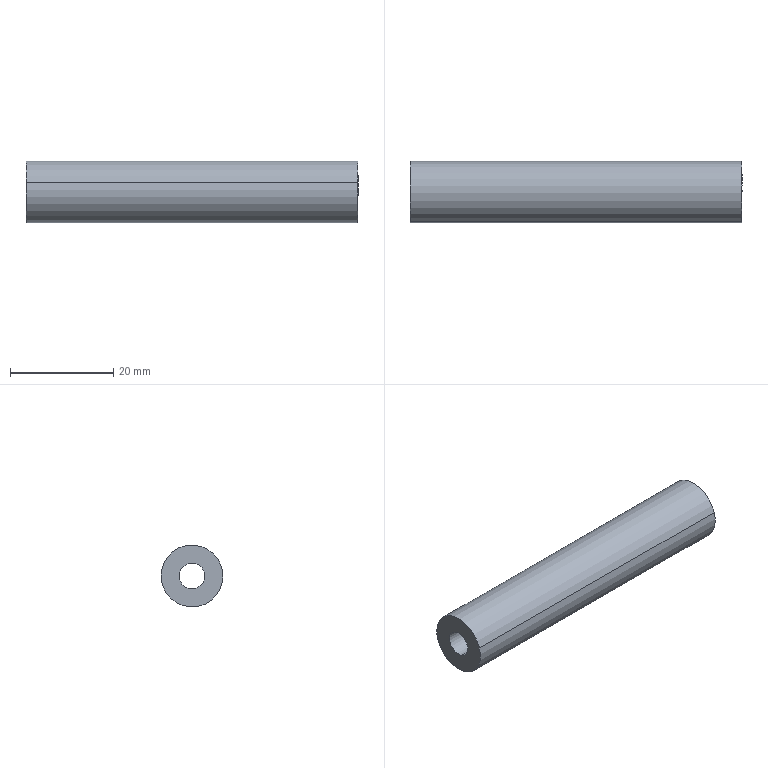Part | STEP file | Completa.sldasm-Part-5_Valor predeterminado | 1 solid | 6 faces | box 64.439 x 12 x 12 mm | volume 6023 mm3 | cylinder 4 | plane 2 | commonest cylinder face diameters 5 x2 12 x2
STEP:
#1=CARTESIAN_POINT('',(0.,0.,0.));
#2=DIRECTION('',(0.,0.,1.));
#3=DIRECTION('',(1.,0.,0.));
#4=AXIS2_PLACEMENT_3D('',#1,#2,#3);
#5=CARTESIAN_POINT('',(-262.606,26.635,-33.219));
#6=VERTEX_POINT('',#5);
#7=CARTESIAN_POINT('',(-198.167,26.635,-33.219));
#8=VERTEX_POINT('',#7);
#9=CARTESIAN_POINT('',(-262.606,26.635,-33.219));
#10=DIRECTION('',(1.,0.,0.));
#11=VECTOR('',#10,1.);
#12=LINE('',#9,#11);
#13=CARTESIAN_POINT('',(-262.606,25.863,-35.597));
#14=DIRECTION('',(1.,0.,0.));
#15=DIRECTION('',(0.,0.309,0.9511));
#16=AXIS2_PLACEMENT_3D('',#13,#14,#15);
#17=CYLINDRICAL_SURFACE('',#16,2.5);
#18=CARTESIAN_POINT('',(6.283,0.));
#19=DIRECTION('',(0.,1.));
#20=VECTOR('',#19,1.);
#21=LINE('',#18,#20);
#22=(GEOMETRIC_REPRESENTATION_CONTEXT(2)PARAMETRIC_REPRESENTATION_CONTEXT()REPRESENTATION_CONTEXT('',''));
#23=DEFINITIONAL_REPRESENTATION('',(#21),#22);
#24=PCURVE('',#17,#23);
#25=CARTESIAN_POINT('',(-262.606,25.863,-35.597));
#26=DIRECTION('',(1.,0.,0.));
#27=DIRECTION('',(0.,0.309,0.9511));
#28=AXIS2_PLACEMENT_3D('',#25,#26,#27);
#29=CYLINDRICAL_SURFACE('',#28,2.5);
#30=CARTESIAN_POINT('',(0.,0.));
#31=DIRECTION('',(0.,1.));
#32=VECTOR('',#31,1.);
#33=LINE('',#30,#32);
#34=(GEOMETRIC_REPRESENTATION_CONTEXT(2)PARAMETRIC_REPRESENTATION_CONTEXT()REPRESENTATION_CONTEXT('',''));
#35=DEFINITIONAL_REPRESENTATION('',(#33),#34);
#36=PCURVE('',#29,#35);
#37=SURFACE_CURVE('',#12,(#24,#36),.PCURVE_S1.);
#38=EDGE_CURVE('',#6,#8,#37,.T.);
#39=ORIENTED_EDGE('',*,*,#38,.T.);
#40=CARTESIAN_POINT('',(-198.167,25.09,-37.974));
#41=VERTEX_POINT('',#40);
#42=CARTESIAN_POINT('',(-198.167,25.863,-35.597));
#43=DIRECTION('',(-1.,0.,0.));
#44=DIRECTION('',(0.,-0.309,-0.9511));
#45=AXIS2_PLACEMENT_3D('',#42,#43,#44);
#46=CIRCLE('',#45,2.5);
#47=CARTESIAN_POINT('',(9.425,64.439));
#48=DIRECTION('',(-1.,0.));
#49=VECTOR('',#48,1.);
#50=LINE('',#47,#49);
#51=(GEOMETRIC_REPRESENTATION_CONTEXT(2)PARAMETRIC_REPRESENTATION_CONTEXT()REPRESENTATION_CONTEXT('',''));
#52=DEFINITIONAL_REPRESENTATION('',(#50),#51);
#53=PCURVE('',#17,#52);
#54=CARTESIAN_POINT('',(-198.167,-9.156,-28.181));
#55=DIRECTION('',(1.,0.,0.));
#56=DIRECTION('',(0.,0.9511,-0.309));
#57=AXIS2_PLACEMENT_3D('',#54,#55,#56);
#58=PLANE('',#57);
#59=CARTESIAN_POINT('',(35.597,1.268));
#60=CARTESIAN_POINT('',(31.267,1.268));
#61=CARTESIAN_POINT('',(33.432,5.018));
#62=CARTESIAN_POINT('',(35.597,8.768));
#63=CARTESIAN_POINT('',(37.762,5.018));
#64=CARTESIAN_POINT('',(39.927,1.268));
#65=CARTESIAN_POINT('',(35.597,1.268));
#66=(BOUNDED_CURVE()B_SPLINE_CURVE(2,(#59,#60,#61,#62,#63,#64,#65),.UNSPECIFIED.,.T.,.F.)B_SPLINE_CURVE_WITH_KNOTS((1,2,2,2,2,1),(-2.094,0.,2.094,4.189,6.283,8.378),.UNSPECIFIED.)CURVE()GEOMETRIC_REPRESENTATION_ITEM()RATIONAL_B_SPLINE_CURVE((1.,0.5,1.,0.5,1.,0.5,1.))REPRESENTATION_ITEM(''));
#67=(GEOMETRIC_REPRESENTATION_CONTEXT(2)PARAMETRIC_REPRESENTATION_CONTEXT()REPRESENTATION_CONTEXT('',''));
#68=DEFINITIONAL_REPRESENTATION('',(#66),#67);
#69=PCURVE('',#58,#68);
#70=SURFACE_CURVE('',#46,(#53,#69),.PCURVE_S1.);
#71=EDGE_CURVE('',#8,#41,#70,.T.);
#72=ORIENTED_EDGE('',*,*,#71,.T.);
#73=CARTESIAN_POINT('',(-262.606,25.09,-37.974));
#74=VERTEX_POINT('',#73);
#75=CARTESIAN_POINT('',(-262.606,25.09,-37.974));
#76=DIRECTION('',(1.,0.,0.));
#77=VECTOR('',#76,1.);
#78=LINE('',#75,#77);
#79=CARTESIAN_POINT('',(3.142,0.));
#80=DIRECTION('',(0.,1.));
#81=VECTOR('',#80,1.);
#82=LINE('',#79,#81);
#83=(GEOMETRIC_REPRESENTATION_CONTEXT(2)PARAMETRIC_REPRESENTATION_CONTEXT()REPRESENTATION_CONTEXT('',''));
#84=DEFINITIONAL_REPRESENTATION('',(#82),#83);
#85=PCURVE('',#17,#84);
#86=CARTESIAN_POINT('',(3.142,0.));
#87=DIRECTION('',(0.,1.));
#88=VECTOR('',#87,1.);
#89=LINE('',#86,#88);
#90=(GEOMETRIC_REPRESENTATION_CONTEXT(2)PARAMETRIC_REPRESENTATION_CONTEXT()REPRESENTATION_CONTEXT('',''));
#91=DEFINITIONAL_REPRESENTATION('',(#89),#90);
#92=PCURVE('',#29,#91);
#93=SURFACE_CURVE('',#78,(#85,#92),.PCURVE_S1.);
#94=EDGE_CURVE('',#74,#41,#93,.T.);
#95=ORIENTED_EDGE('',*,*,#94,.F.);
#96=CARTESIAN_POINT('',(-262.606,25.863,-35.597));
#97=DIRECTION('',(-1.,0.,0.));
#98=DIRECTION('',(0.,-0.309,-0.9511));
#99=AXIS2_PLACEMENT_3D('',#96,#97,#98);
#100=CIRCLE('',#99,2.5);
#101=CARTESIAN_POINT('',(9.425,0.));
#102=DIRECTION('',(-1.,0.));
#103=VECTOR('',#102,1.);
#104=LINE('',#101,#103);
#105=(GEOMETRIC_REPRESENTATION_CONTEXT(2)PARAMETRIC_REPRESENTATION_CONTEXT()REPRESENTATION_CONTEXT('',''));
#106=DEFINITIONAL_REPRESENTATION('',(#104),#105);
#107=PCURVE('',#17,#106);
#108=CARTESIAN_POINT('',(-262.606,25.863,-35.597));
#109=DIRECTION('',(1.,0.,0.));
#110=DIRECTION('',(0.,0.9511,-0.309));
#111=AXIS2_PLACEMENT_3D('',#108,#109,#110);
#112=PLANE('',#111);
#113=CARTESIAN_POINT('',(0.,-2.5));
#114=CARTESIAN_POINT('',(-4.33,-2.5));
#115=CARTESIAN_POINT('',(-2.165,1.25));
#116=CARTESIAN_POINT('',(0.,5.));
#117=CARTESIAN_POINT('',(2.165,1.25));
#118=CARTESIAN_POINT('',(4.33,-2.5));
#119=CARTESIAN_POINT('',(0.,-2.5));
#120=(BOUNDED_CURVE()B_SPLINE_CURVE(2,(#113,#114,#115,#116,#117,#118,#119),.UNSPECIFIED.,.T.,.F.)B_SPLINE_CURVE_WITH_KNOTS((1,2,2,2,2,1),(-2.094,0.,2.094,4.189,6.283,8.378),.UNSPECIFIED.)CURVE()GEOMETRIC_REPRESENTATION_ITEM()RATIONAL_B_SPLINE_CURVE((1.,0.5,1.,0.5,1.,0.5,1.))REPRESENTATION_ITEM(''));
#121=(GEOMETRIC_REPRESENTATION_CONTEXT(2)PARAMETRIC_REPRESENTATION_CONTEXT()REPRESENTATION_CONTEXT('',''));
#122=DEFINITIONAL_REPRESENTATION('',(#120),#121);
#123=PCURVE('',#112,#122);
#124=SURFACE_CURVE('',#100,(#107,#123),.PCURVE_S1.);
#125=EDGE_CURVE('',#6,#74,#124,.T.);
#126=ORIENTED_EDGE('',*,*,#125,.F.);
#127=EDGE_LOOP('',(#39,#72,#95,#126));
#128=FACE_BOUND('',#127,.F.);
#129=ADVANCED_FACE('',(#128),#17,.F.);
#130=CARTESIAN_POINT('',(-198.167,31.569,-37.451));
#131=VERTEX_POINT('',#130);
#132=CARTESIAN_POINT('',(-198.167,20.156,-33.743));
#133=VERTEX_POINT('',#132);
#134=CARTESIAN_POINT('',(-198.167,25.863,-35.597));
#135=DIRECTION('',(1.,0.,0.));
#136=DIRECTION('',(0.,0.9511,-0.309));
#137=AXIS2_PLACEMENT_3D('',#134,#135,#136);
#138=CIRCLE('',#137,6.);
#139=CARTESIAN_POINT('',(-72.606,25.863,-35.597));
#140=DIRECTION('',(-1.,0.,0.));
#141=DIRECTION('',(0.,-0.9511,0.309));
#142=AXIS2_PLACEMENT_3D('',#139,#140,#141);
#143=CYLINDRICAL_SURFACE('',#142,6.);
#144=CARTESIAN_POINT('',(3.142,125.561));
#145=DIRECTION('',(-1.,0.));
#146=VECTOR('',#145,1.);
#147=LINE('',#144,#146);
#148=(GEOMETRIC_REPRESENTATION_CONTEXT(2)PARAMETRIC_REPRESENTATION_CONTEXT()REPRESENTATION_CONTEXT('',''));
#149=DEFINITIONAL_REPRESENTATION('',(#147),#148);
#150=PCURVE('',#143,#149);
#151=CARTESIAN_POINT('',(35.597,3.768));
#152=DIRECTION('',(1.,0.));
#153=AXIS2_PLACEMENT_2D('',#151,#152);
#154=CIRCLE('',#153,6.);
#155=(GEOMETRIC_REPRESENTATION_CONTEXT(2)PARAMETRIC_REPRESENTATION_CONTEXT()REPRESENTATION_CONTEXT('',''));
#156=DEFINITIONAL_REPRESENTATION('',(#154),#155);
#157=PCURVE('',#58,#156);
#158=SURFACE_CURVE('',#138,(#150,#157),.PCURVE_S1.);
#159=EDGE_CURVE('',#131,#133,#158,.T.);
#160=ORIENTED_EDGE('',*,*,#159,.F.);
#161=CARTESIAN_POINT('',(-262.606,31.569,-37.451));
#162=VERTEX_POINT('',#161);
#163=CARTESIAN_POINT('',(-72.606,31.569,-37.451));
#164=DIRECTION('',(-1.,0.,0.));
#165=VECTOR('',#164,1.);
#166=LINE('',#163,#165);
#167=CARTESIAN_POINT('',(3.142,0.));
#168=DIRECTION('',(0.,1.));
#169=VECTOR('',#168,1.);
#170=LINE('',#167,#169);
#171=(GEOMETRIC_REPRESENTATION_CONTEXT(2)PARAMETRIC_REPRESENTATION_CONTEXT()REPRESENTATION_CONTEXT('',''));
#172=DEFINITIONAL_REPRESENTATION('',(#170),#171);
#173=PCURVE('',#143,#172);
#174=CARTESIAN_POINT('',(-72.606,25.863,-35.597));
#175=DIRECTION('',(-1.,0.,0.));
#176=DIRECTION('',(0.,-0.9511,0.309));
#177=AXIS2_PLACEMENT_3D('',#174,#175,#176);
#178=CYLINDRICAL_SURFACE('',#177,6.);
#179=CARTESIAN_POINT('',(3.142,0.));
#180=DIRECTION('',(0.,1.));
#181=VECTOR('',#180,1.);
#182=LINE('',#179,#181);
#183=(GEOMETRIC_REPRESENTATION_CONTEXT(2)PARAMETRIC_REPRESENTATION_CONTEXT()REPRESENTATION_CONTEXT('',''));
#184=DEFINITIONAL_REPRESENTATION('',(#182),#183);
#185=PCURVE('',#178,#184);
#186=SURFACE_CURVE('',#166,(#173,#185),.PCURVE_S1.);
#187=EDGE_CURVE('',#131,#162,#186,.T.);
#188=ORIENTED_EDGE('',*,*,#187,.T.);
#189=CARTESIAN_POINT('',(-262.606,20.156,-33.743));
#190=VERTEX_POINT('',#189);
#191=CARTESIAN_POINT('',(-262.606,25.863,-35.597));
#192=DIRECTION('',(1.,0.,0.));
#193=DIRECTION('',(0.,-0.9511,0.309));
#194=AXIS2_PLACEMENT_3D('',#191,#192,#193);
#195=CIRCLE('',#194,6.);
#196=CARTESIAN_POINT('',(6.283,190.));
#197=DIRECTION('',(-1.,0.));
#198=VECTOR('',#197,1.);
#199=LINE('',#196,#198);
#200=(GEOMETRIC_REPRESENTATION_CONTEXT(2)PARAMETRIC_REPRESENTATION_CONTEXT()REPRESENTATION_CONTEXT('',''));
#201=DEFINITIONAL_REPRESENTATION('',(#199),#200);
#202=PCURVE('',#143,#201);
#203=CARTESIAN_POINT('',(0.,0.));
#204=DIRECTION('',(-1.,0.));
#205=AXIS2_PLACEMENT_2D('',#203,#204);
#206=CIRCLE('',#205,6.);
#207=(GEOMETRIC_REPRESENTATION_CONTEXT(2)PARAMETRIC_REPRESENTATION_CONTEXT()REPRESENTATION_CONTEXT('',''));
#208=DEFINITIONAL_REPRESENTATION('',(#206),#207);
#209=PCURVE('',#112,#208);
#210=SURFACE_CURVE('',#195,(#202,#209),.PCURVE_S1.);
#211=EDGE_CURVE('',#162,#190,#210,.T.);
#212=ORIENTED_EDGE('',*,*,#211,.T.);
#213=CARTESIAN_POINT('',(-72.606,20.156,-33.743));
#214=DIRECTION('',(-1.,0.,0.));
#215=VECTOR('',#214,1.);
#216=LINE('',#213,#215);
#217=CARTESIAN_POINT('',(0.,0.));
#218=DIRECTION('',(0.,1.));
#219=VECTOR('',#218,1.);
#220=LINE('',#217,#219);
#221=(GEOMETRIC_REPRESENTATION_CONTEXT(2)PARAMETRIC_REPRESENTATION_CONTEXT()REPRESENTATION_CONTEXT('',''));
#222=DEFINITIONAL_REPRESENTATION('',(#220),#221);
#223=PCURVE('',#143,#222);
#224=CARTESIAN_POINT('',(6.283,0.));
#225=DIRECTION('',(0.,1.));
#226=VECTOR('',#225,1.);
#227=LINE('',#224,#226);
#228=(GEOMETRIC_REPRESENTATION_CONTEXT(2)PARAMETRIC_REPRESENTATION_CONTEXT()REPRESENTATION_CONTEXT('',''));
#229=DEFINITIONAL_REPRESENTATION('',(#227),#228);
#230=PCURVE('',#178,#229);
#231=SURFACE_CURVE('',#216,(#223,#230),.PCURVE_S1.);
#232=EDGE_CURVE('',#133,#190,#231,.T.);
#233=ORIENTED_EDGE('',*,*,#232,.F.);
#234=EDGE_LOOP('',(#160,#188,#212,#233));
#235=FACE_BOUND('',#234,.T.);
#236=ADVANCED_FACE('',(#235),#143,.T.);
#237=CARTESIAN_POINT('',(-262.606,25.863,-35.597));
#238=DIRECTION('',(1.,0.,0.));
#239=DIRECTION('',(0.,-0.9511,0.309));
#240=AXIS2_PLACEMENT_3D('',#237,#238,#239);
#241=CIRCLE('',#240,6.);
#242=CARTESIAN_POINT('',(0.,0.));
#243=DIRECTION('',(-1.,0.));
#244=AXIS2_PLACEMENT_2D('',#242,#243);
#245=CIRCLE('',#244,6.);
#246=(GEOMETRIC_REPRESENTATION_CONTEXT(2)PARAMETRIC_REPRESENTATION_CONTEXT()REPRESENTATION_CONTEXT('',''));
#247=DEFINITIONAL_REPRESENTATION('',(#245),#246);
#248=PCURVE('',#112,#247);
#249=CARTESIAN_POINT('',(6.283,190.));
#250=DIRECTION('',(-1.,0.));
#251=VECTOR('',#250,1.);
#252=LINE('',#249,#251);
#253=(GEOMETRIC_REPRESENTATION_CONTEXT(2)PARAMETRIC_REPRESENTATION_CONTEXT()REPRESENTATION_CONTEXT('',''));
#254=DEFINITIONAL_REPRESENTATION('',(#252),#253);
#255=PCURVE('',#178,#254);
#256=SURFACE_CURVE('',#241,(#248,#255),.PCURVE_S1.);
#257=EDGE_CURVE('',#190,#162,#256,.T.);
#258=ORIENTED_EDGE('',*,*,#257,.F.);
#259=ORIENTED_EDGE('',*,*,#211,.F.);
#260=EDGE_LOOP('',(#258,#259));
#261=FACE_BOUND('',#260,.T.);
#262=ORIENTED_EDGE('',*,*,#125,.F.);
#263=CARTESIAN_POINT('',(-262.606,25.863,-35.597));
#264=DIRECTION('',(-1.,0.,0.));
#265=DIRECTION('',(0.,-0.309,-0.9511));
#266=AXIS2_PLACEMENT_3D('',#263,#264,#265);
#267=CIRCLE('',#266,2.5);
#268=CARTESIAN_POINT('',(0.,-2.5));
#269=CARTESIAN_POINT('',(-4.33,-2.5));
#270=CARTESIAN_POINT('',(-2.165,1.25));
#271=CARTESIAN_POINT('',(0.,5.));
#272=CARTESIAN_POINT('',(2.165,1.25));
#273=CARTESIAN_POINT('',(4.33,-2.5));
#274=CARTESIAN_POINT('',(0.,-2.5));
#275=(BOUNDED_CURVE()B_SPLINE_CURVE(2,(#268,#269,#270,#271,#272,#273,#274),.UNSPECIFIED.,.T.,.F.)B_SPLINE_CURVE_WITH_KNOTS((1,2,2,2,2,1),(-2.094,0.,2.094,4.189,6.283,8.378),.UNSPECIFIED.)CURVE()GEOMETRIC_REPRESENTATION_ITEM()RATIONAL_B_SPLINE_CURVE((1.,0.5,1.,0.5,1.,0.5,1.))REPRESENTATION_ITEM(''));
#276=(GEOMETRIC_REPRESENTATION_CONTEXT(2)PARAMETRIC_REPRESENTATION_CONTEXT()REPRESENTATION_CONTEXT('',''));
#277=DEFINITIONAL_REPRESENTATION('',(#275),#276);
#278=PCURVE('',#112,#277);
#279=CARTESIAN_POINT('',(3.142,0.));
#280=DIRECTION('',(-1.,0.));
#281=VECTOR('',#280,1.);
#282=LINE('',#279,#281);
#283=(GEOMETRIC_REPRESENTATION_CONTEXT(2)PARAMETRIC_REPRESENTATION_CONTEXT()REPRESENTATION_CONTEXT('',''));
#284=DEFINITIONAL_REPRESENTATION('',(#282),#283);
#285=PCURVE('',#29,#284);
#286=SURFACE_CURVE('',#267,(#278,#285),.PCURVE_S1.);
#287=EDGE_CURVE('',#74,#6,#286,.T.);
#288=ORIENTED_EDGE('',*,*,#287,.F.);
#289=EDGE_LOOP('',(#262,#288));
#290=FACE_BOUND('',#289,.T.);
#291=ADVANCED_FACE('',(#261,#290),#112,.F.);
#292=CARTESIAN_POINT('',(-198.167,25.863,-35.597));
#293=DIRECTION('',(1.,0.,0.));
#294=DIRECTION('',(0.,0.9511,-0.309));
#295=AXIS2_PLACEMENT_3D('',#292,#293,#294);
#296=CIRCLE('',#295,6.);
#297=CARTESIAN_POINT('',(35.597,3.768));
#298=DIRECTION('',(1.,0.));
#299=AXIS2_PLACEMENT_2D('',#297,#298);
#300=CIRCLE('',#299,6.);
#301=(GEOMETRIC_REPRESENTATION_CONTEXT(2)PARAMETRIC_REPRESENTATION_CONTEXT()REPRESENTATION_CONTEXT('',''));
#302=DEFINITIONAL_REPRESENTATION('',(#300),#301);
#303=PCURVE('',#58,#302);
#304=CARTESIAN_POINT('',(9.425,125.561));
#305=DIRECTION('',(-1.,0.));
#306=VECTOR('',#305,1.);
#307=LINE('',#304,#306);
#308=(GEOMETRIC_REPRESENTATION_CONTEXT(2)PARAMETRIC_REPRESENTATION_CONTEXT()REPRESENTATION_CONTEXT('',''));
#309=DEFINITIONAL_REPRESENTATION('',(#307),#308);
#310=PCURVE('',#178,#309);
#311=SURFACE_CURVE('',#296,(#303,#310),.PCURVE_S1.);
#312=EDGE_CURVE('',#133,#131,#311,.T.);
#313=ORIENTED_EDGE('',*,*,#312,.T.);
#314=ORIENTED_EDGE('',*,*,#159,.T.);
#315=EDGE_LOOP('',(#313,#314));
#316=FACE_BOUND('',#315,.T.);
#317=ORIENTED_EDGE('',*,*,#71,.T.);
#318=CARTESIAN_POINT('',(-198.167,25.863,-35.597));
#319=DIRECTION('',(-1.,0.,0.));
#320=DIRECTION('',(0.,-0.309,-0.9511));
#321=AXIS2_PLACEMENT_3D('',#318,#319,#320);
#322=CIRCLE('',#321,2.5);
#323=CARTESIAN_POINT('',(35.597,1.268));
#324=CARTESIAN_POINT('',(31.267,1.268));
#325=CARTESIAN_POINT('',(33.432,5.018));
#326=CARTESIAN_POINT('',(35.597,8.768));
#327=CARTESIAN_POINT('',(37.762,5.018));
#328=CARTESIAN_POINT('',(39.927,1.268));
#329=CARTESIAN_POINT('',(35.597,1.268));
#330=(BOUNDED_CURVE()B_SPLINE_CURVE(2,(#323,#324,#325,#326,#327,#328,#329),.UNSPECIFIED.,.T.,.F.)B_SPLINE_CURVE_WITH_KNOTS((1,2,2,2,2,1),(-2.094,0.,2.094,4.189,6.283,8.378),.UNSPECIFIED.)CURVE()GEOMETRIC_REPRESENTATION_ITEM()RATIONAL_B_SPLINE_CURVE((1.,0.5,1.,0.5,1.,0.5,1.))REPRESENTATION_ITEM(''));
#331=(GEOMETRIC_REPRESENTATION_CONTEXT(2)PARAMETRIC_REPRESENTATION_CONTEXT()REPRESENTATION_CONTEXT('',''));
#332=DEFINITIONAL_REPRESENTATION('',(#330),#331);
#333=PCURVE('',#58,#332);
#334=CARTESIAN_POINT('',(3.142,64.439));
#335=DIRECTION('',(-1.,0.));
#336=VECTOR('',#335,1.);
#337=LINE('',#334,#336);
#338=(GEOMETRIC_REPRESENTATION_CONTEXT(2)PARAMETRIC_REPRESENTATION_CONTEXT()REPRESENTATION_CONTEXT('',''));
#339=DEFINITIONAL_REPRESENTATION('',(#337),#338);
#340=PCURVE('',#29,#339);
#341=SURFACE_CURVE('',#322,(#333,#340),.PCURVE_S1.);
#342=EDGE_CURVE('',#41,#8,#341,.T.);
#343=ORIENTED_EDGE('',*,*,#342,.T.);
#344=EDGE_LOOP('',(#317,#343));
#345=FACE_BOUND('',#344,.T.);
#346=ADVANCED_FACE('',(#316,#345),#58,.T.);
#347=ORIENTED_EDGE('',*,*,#187,.F.);
#348=ORIENTED_EDGE('',*,*,#312,.F.);
#349=ORIENTED_EDGE('',*,*,#232,.T.);
#350=ORIENTED_EDGE('',*,*,#257,.T.);
#351=EDGE_LOOP('',(#347,#348,#349,#350));
#352=FACE_BOUND('',#351,.T.);
#353=ADVANCED_FACE('',(#352),#178,.T.);
#354=ORIENTED_EDGE('',*,*,#342,.T.);
#355=ORIENTED_EDGE('',*,*,#38,.F.);
#356=ORIENTED_EDGE('',*,*,#287,.F.);
#357=ORIENTED_EDGE('',*,*,#94,.T.);
#358=EDGE_LOOP('',(#354,#355,#356,#357));
#359=FACE_BOUND('',#358,.F.);
#360=ADVANCED_FACE('',(#359),#29,.F.);
#361=CLOSED_SHELL('',(#129,#236,#291,#346,#353,#360));
#362=MANIFOLD_SOLID_BREP('',#361);
#363=(LENGTH_UNIT()NAMED_UNIT(*)SI_UNIT(.MILLI.,.METRE.));
#364=UNCERTAINTY_MEASURE_WITH_UNIT(LENGTH_MEASURE(0.0000001),#363,'','');
#365=(NAMED_UNIT(*)PLANE_ANGLE_UNIT()SI_UNIT($,.RADIAN.));
#366=(NAMED_UNIT(*)SI_UNIT($,.STERADIAN.)SOLID_ANGLE_UNIT());
#367=(GEOMETRIC_REPRESENTATION_CONTEXT(3)GLOBAL_UNCERTAINTY_ASSIGNED_CONTEXT((#364))GLOBAL_UNIT_ASSIGNED_CONTEXT((#363,#365,#366))REPRESENTATION_CONTEXT('',''));
#368=ADVANCED_BREP_SHAPE_REPRESENTATION('',(#4,#362),#367);